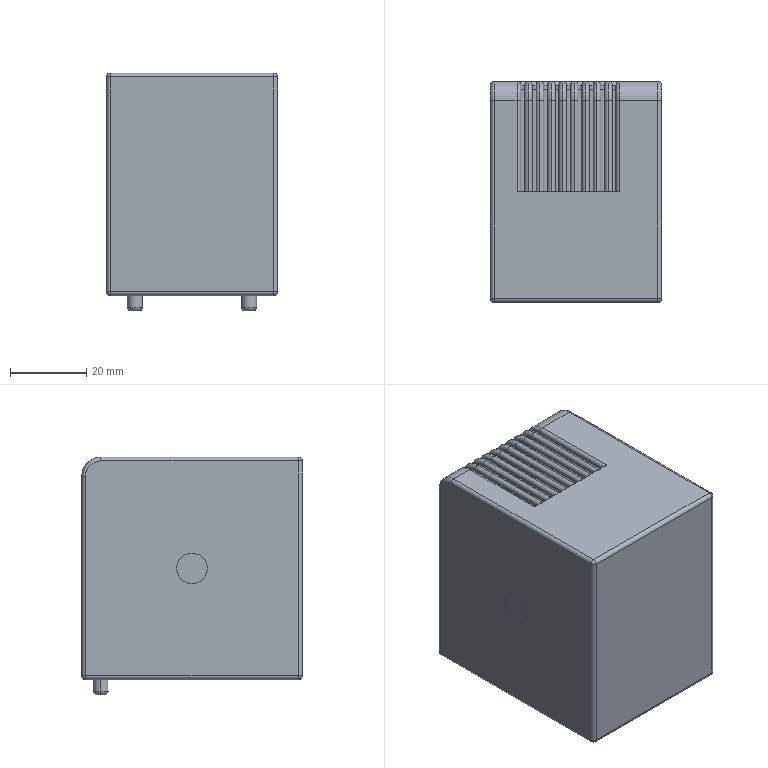Part | STEP file | Mirrored MJ45 motor support seat | 1 solid | 222 faces | box 45 x 58 x 62.5 mm | volume 148250 mm3 | plane 88 | cylinder 78 | torus 42 | cone 8 | sphere 6 | commonest cylinder face diameters 2 x56 4.2 x8 5.5 x6 4 x4 10 x2 16 x2